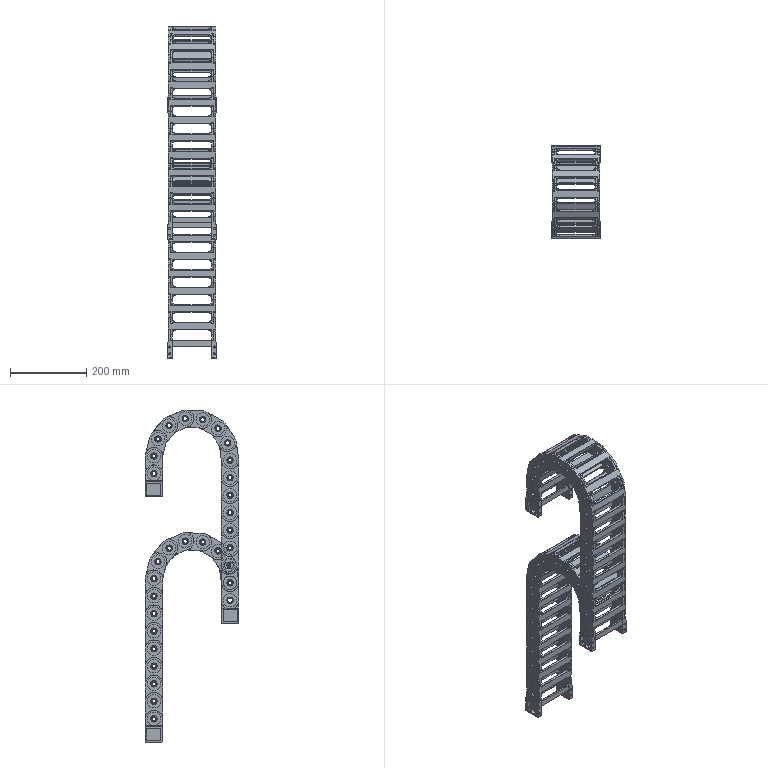Part | SolidWorks | features BaseBody 18, LPattern 4 | 34 solids | 8662 faces | volume 2054187 mm3 | cylinder 5418 | plane 3244 | commonest cylinder face diameters 2 x912 1 x620 4 x390 20.12 x330 41.64 x310 17.1 x264